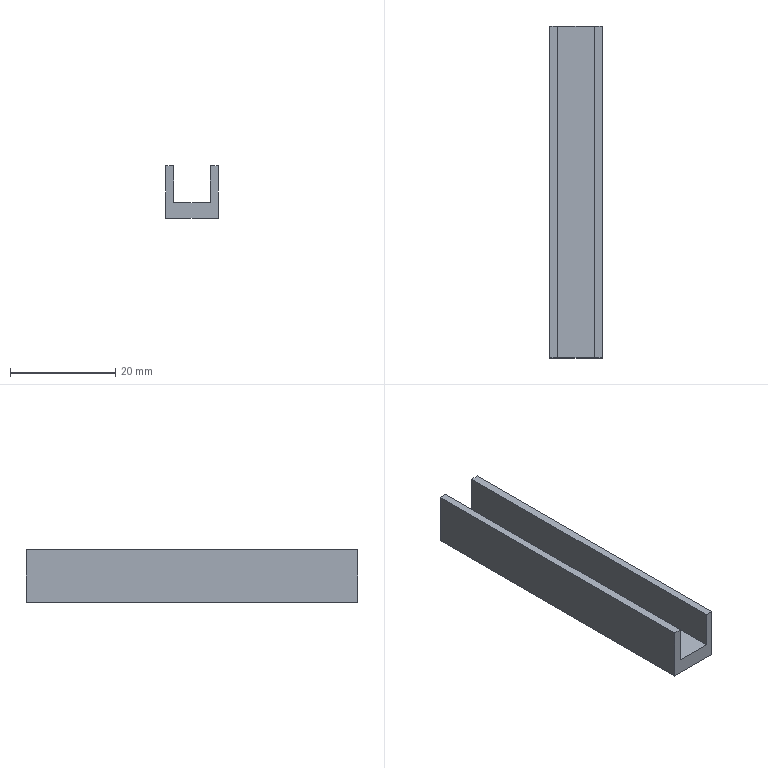Part | STEP file | Magazine box | 1 solid | 10 faces | box 10 x 63 x 10 mm | volume 3213 mm3 | plane 10
STEP:
#1=CARTESIAN_POINT('',(5.,31.5,5.));
#2=VERTEX_POINT('',#1);
#3=CARTESIAN_POINT('',(3.5,31.5,5.));
#4=VERTEX_POINT('',#3);
#5=CARTESIAN_POINT('',(-5.,31.5,5.));
#6=DIRECTION('',(-1.,0.,0.));
#7=VECTOR('',#6,1000.);
#8=LINE('',#5,#7);
#9=EDGE_CURVE('',#2,#4,#8,.T.);
#10=ORIENTED_EDGE('',*,*,#9,.T.);
#11=CARTESIAN_POINT('',(3.5,-31.5,5.));
#12=VERTEX_POINT('',#11);
#13=CARTESIAN_POINT('',(3.5,0.,5.));
#14=DIRECTION('',(0.,-1.,0.));
#15=VECTOR('',#14,1000.);
#16=LINE('',#13,#15);
#17=EDGE_CURVE('',#4,#12,#16,.T.);
#18=ORIENTED_EDGE('',*,*,#17,.T.);
#19=CARTESIAN_POINT('',(5.,-31.5,5.));
#20=VERTEX_POINT('',#19);
#21=CARTESIAN_POINT('',(-5.,-31.5,5.));
#22=DIRECTION('',(1.,0.,0.));
#23=VECTOR('',#22,1000.);
#24=LINE('',#21,#23);
#25=EDGE_CURVE('',#12,#20,#24,.T.);
#26=ORIENTED_EDGE('',*,*,#25,.T.);
#27=CARTESIAN_POINT('',(5.,-31.5,5.));
#28=DIRECTION('',(0.,1.,0.));
#29=VECTOR('',#28,1000.);
#30=LINE('',#27,#29);
#31=EDGE_CURVE('',#20,#2,#30,.T.);
#32=ORIENTED_EDGE('',*,*,#31,.T.);
#33=EDGE_LOOP('',(#10,#18,#26,#32));
#34=FACE_OUTER_BOUND('',#33,.T.);
#35=CARTESIAN_POINT('',(0.,0.,5.));
#36=DIRECTION('',(0.,0.,-1.));
#37=DIRECTION('',(-1.,0.,0.));
#38=AXIS2_PLACEMENT_3D('',#35,#36,#37);
#39=PLANE('',#38);
#40=ADVANCED_FACE('',(#34),#39,.F.);
#41=CARTESIAN_POINT('',(5.,-31.5,-5.));
#42=VERTEX_POINT('',#41);
#43=CARTESIAN_POINT('',(5.,31.5,-5.));
#44=VERTEX_POINT('',#43);
#45=CARTESIAN_POINT('',(5.,-31.5,-5.));
#46=DIRECTION('',(0.,1.,0.));
#47=VECTOR('',#46,1000.);
#48=LINE('',#45,#47);
#49=EDGE_CURVE('',#42,#44,#48,.T.);
#50=ORIENTED_EDGE('',*,*,#49,.T.);
#51=CARTESIAN_POINT('',(5.,31.5,5.));
#52=DIRECTION('',(0.,0.,-1.));
#53=VECTOR('',#52,1000.);
#54=LINE('',#51,#53);
#55=EDGE_CURVE('',#2,#44,#54,.T.);
#56=ORIENTED_EDGE('',*,*,#55,.F.);
#57=ORIENTED_EDGE('',*,*,#31,.F.);
#58=CARTESIAN_POINT('',(5.,-31.5,5.));
#59=DIRECTION('',(0.,0.,-1.));
#60=VECTOR('',#59,1000.);
#61=LINE('',#58,#60);
#62=EDGE_CURVE('',#20,#42,#61,.T.);
#63=ORIENTED_EDGE('',*,*,#62,.T.);
#64=EDGE_LOOP('',(#50,#56,#57,#63));
#65=FACE_OUTER_BOUND('',#64,.T.);
#66=CARTESIAN_POINT('',(5.,-31.5,5.));
#67=DIRECTION('',(-1.,0.,0.));
#68=DIRECTION('',(0.,-1.,0.));
#69=AXIS2_PLACEMENT_3D('',#66,#67,#68);
#70=PLANE('',#69);
#71=ADVANCED_FACE('',(#65),#70,.F.);
#72=CARTESIAN_POINT('',(3.5,31.5,-2.));
#73=VERTEX_POINT('',#72);
#74=CARTESIAN_POINT('',(-3.5,31.5,-2.));
#75=VERTEX_POINT('',#74);
#76=CARTESIAN_POINT('',(-5.,31.5,-2.));
#77=DIRECTION('',(-1.,0.,0.));
#78=VECTOR('',#77,1000.);
#79=LINE('',#76,#78);
#80=EDGE_CURVE('',#73,#75,#79,.T.);
#81=ORIENTED_EDGE('',*,*,#80,.F.);
#82=CARTESIAN_POINT('',(3.5,31.5,5.));
#83=DIRECTION('',(0.,0.,1.));
#84=VECTOR('',#83,1000.);
#85=LINE('',#82,#84);
#86=EDGE_CURVE('',#73,#4,#85,.T.);
#87=ORIENTED_EDGE('',*,*,#86,.T.);
#88=ORIENTED_EDGE('',*,*,#9,.F.);
#89=ORIENTED_EDGE('',*,*,#55,.T.);
#90=CARTESIAN_POINT('',(-5.,31.5,-5.));
#91=VERTEX_POINT('',#90);
#92=CARTESIAN_POINT('',(-5.,31.5,-5.));
#93=DIRECTION('',(-1.,0.,0.));
#94=VECTOR('',#93,1000.);
#95=LINE('',#92,#94);
#96=EDGE_CURVE('',#44,#91,#95,.T.);
#97=ORIENTED_EDGE('',*,*,#96,.T.);
#98=CARTESIAN_POINT('',(-5.,31.5,5.));
#99=VERTEX_POINT('',#98);
#100=CARTESIAN_POINT('',(-5.,31.5,5.));
#101=DIRECTION('',(0.,0.,-1.));
#102=VECTOR('',#101,1000.);
#103=LINE('',#100,#102);
#104=EDGE_CURVE('',#99,#91,#103,.T.);
#105=ORIENTED_EDGE('',*,*,#104,.F.);
#106=CARTESIAN_POINT('',(-3.5,31.5,5.));
#107=VERTEX_POINT('',#106);
#108=CARTESIAN_POINT('',(-5.,31.5,5.));
#109=DIRECTION('',(-1.,0.,0.));
#110=VECTOR('',#109,1000.);
#111=LINE('',#108,#110);
#112=EDGE_CURVE('',#107,#99,#111,.T.);
#113=ORIENTED_EDGE('',*,*,#112,.F.);
#114=CARTESIAN_POINT('',(-3.5,31.5,5.));
#115=DIRECTION('',(0.,0.,-1.));
#116=VECTOR('',#115,1000.);
#117=LINE('',#114,#116);
#118=EDGE_CURVE('',#107,#75,#117,.T.);
#119=ORIENTED_EDGE('',*,*,#118,.T.);
#120=EDGE_LOOP('',(#81,#87,#88,#89,#97,#105,#113,#119));
#121=FACE_OUTER_BOUND('',#120,.T.);
#122=CARTESIAN_POINT('',(-5.,31.5,5.));
#123=DIRECTION('',(0.,-1.,0.));
#124=DIRECTION('',(1.,0.,0.));
#125=AXIS2_PLACEMENT_3D('',#122,#123,#124);
#126=PLANE('',#125);
#127=ADVANCED_FACE('',(#121),#126,.F.);
#128=CARTESIAN_POINT('',(-5.,-31.5,-5.));
#129=VERTEX_POINT('',#128);
#130=CARTESIAN_POINT('',(-5.,-31.5,-5.));
#131=DIRECTION('',(0.,-1.,0.));
#132=VECTOR('',#131,1000.);
#133=LINE('',#130,#132);
#134=EDGE_CURVE('',#91,#129,#133,.T.);
#135=ORIENTED_EDGE('',*,*,#134,.T.);
#136=CARTESIAN_POINT('',(-5.,-31.5,5.));
#137=VERTEX_POINT('',#136);
#138=CARTESIAN_POINT('',(-5.,-31.5,5.));
#139=DIRECTION('',(0.,0.,-1.));
#140=VECTOR('',#139,1000.);
#141=LINE('',#138,#140);
#142=EDGE_CURVE('',#137,#129,#141,.T.);
#143=ORIENTED_EDGE('',*,*,#142,.F.);
#144=CARTESIAN_POINT('',(-5.,-31.5,5.));
#145=DIRECTION('',(0.,-1.,0.));
#146=VECTOR('',#145,1000.);
#147=LINE('',#144,#146);
#148=EDGE_CURVE('',#99,#137,#147,.T.);
#149=ORIENTED_EDGE('',*,*,#148,.F.);
#150=ORIENTED_EDGE('',*,*,#104,.T.);
#151=EDGE_LOOP('',(#135,#143,#149,#150));
#152=FACE_OUTER_BOUND('',#151,.T.);
#153=CARTESIAN_POINT('',(-5.,-31.5,5.));
#154=DIRECTION('',(1.,0.,0.));
#155=DIRECTION('',(0.,0.,-1.));
#156=AXIS2_PLACEMENT_3D('',#153,#154,#155);
#157=PLANE('',#156);
#158=ADVANCED_FACE('',(#152),#157,.F.);
#159=ORIENTED_EDGE('',*,*,#25,.F.);
#160=CARTESIAN_POINT('',(3.5,-31.5,-2.));
#161=VERTEX_POINT('',#160);
#162=CARTESIAN_POINT('',(3.5,-31.5,5.));
#163=DIRECTION('',(0.,0.,-1.));
#164=VECTOR('',#163,1000.);
#165=LINE('',#162,#164);
#166=EDGE_CURVE('',#12,#161,#165,.T.);
#167=ORIENTED_EDGE('',*,*,#166,.T.);
#168=CARTESIAN_POINT('',(-3.5,-31.5,-2.));
#169=VERTEX_POINT('',#168);
#170=CARTESIAN_POINT('',(-5.,-31.5,-2.));
#171=DIRECTION('',(1.,0.,0.));
#172=VECTOR('',#171,1000.);
#173=LINE('',#170,#172);
#174=EDGE_CURVE('',#169,#161,#173,.T.);
#175=ORIENTED_EDGE('',*,*,#174,.F.);
#176=CARTESIAN_POINT('',(-3.5,-31.5,5.));
#177=VERTEX_POINT('',#176);
#178=CARTESIAN_POINT('',(-3.5,-31.5,5.));
#179=DIRECTION('',(0.,0.,1.));
#180=VECTOR('',#179,1000.);
#181=LINE('',#178,#180);
#182=EDGE_CURVE('',#169,#177,#181,.T.);
#183=ORIENTED_EDGE('',*,*,#182,.T.);
#184=CARTESIAN_POINT('',(-5.,-31.5,5.));
#185=DIRECTION('',(1.,0.,0.));
#186=VECTOR('',#185,1000.);
#187=LINE('',#184,#186);
#188=EDGE_CURVE('',#137,#177,#187,.T.);
#189=ORIENTED_EDGE('',*,*,#188,.F.);
#190=ORIENTED_EDGE('',*,*,#142,.T.);
#191=CARTESIAN_POINT('',(-5.,-31.5,-5.));
#192=DIRECTION('',(1.,0.,0.));
#193=VECTOR('',#192,1000.);
#194=LINE('',#191,#193);
#195=EDGE_CURVE('',#129,#42,#194,.T.);
#196=ORIENTED_EDGE('',*,*,#195,.T.);
#197=ORIENTED_EDGE('',*,*,#62,.F.);
#198=EDGE_LOOP('',(#159,#167,#175,#183,#189,#190,#196,#197));
#199=FACE_OUTER_BOUND('',#198,.T.);
#200=CARTESIAN_POINT('',(-5.,-31.5,5.));
#201=DIRECTION('',(0.,1.,0.));
#202=DIRECTION('',(0.,0.,1.));
#203=AXIS2_PLACEMENT_3D('',#200,#201,#202);
#204=PLANE('',#203);
#205=ADVANCED_FACE('',(#199),#204,.F.);
#206=ORIENTED_EDGE('',*,*,#188,.T.);
#207=CARTESIAN_POINT('',(-3.5,0.,5.));
#208=DIRECTION('',(0.,1.,0.));
#209=VECTOR('',#208,1000.);
#210=LINE('',#207,#209);
#211=EDGE_CURVE('',#177,#107,#210,.T.);
#212=ORIENTED_EDGE('',*,*,#211,.T.);
#213=ORIENTED_EDGE('',*,*,#112,.T.);
#214=ORIENTED_EDGE('',*,*,#148,.T.);
#215=EDGE_LOOP('',(#206,#212,#213,#214));
#216=FACE_OUTER_BOUND('',#215,.T.);
#217=CARTESIAN_POINT('',(0.,0.,5.));
#218=DIRECTION('',(0.,0.,-1.));
#219=DIRECTION('',(-1.,0.,0.));
#220=AXIS2_PLACEMENT_3D('',#217,#218,#219);
#221=PLANE('',#220);
#222=ADVANCED_FACE('',(#216),#221,.F.);
#223=ORIENTED_EDGE('',*,*,#49,.F.);
#224=ORIENTED_EDGE('',*,*,#195,.F.);
#225=ORIENTED_EDGE('',*,*,#134,.F.);
#226=ORIENTED_EDGE('',*,*,#96,.F.);
#227=EDGE_LOOP('',(#223,#224,#225,#226));
#228=FACE_OUTER_BOUND('',#227,.T.);
#229=CARTESIAN_POINT('',(0.,0.,-5.));
#230=DIRECTION('',(0.,0.,-1.));
#231=DIRECTION('',(-1.,0.,0.));
#232=AXIS2_PLACEMENT_3D('',#229,#230,#231);
#233=PLANE('',#232);
#234=ADVANCED_FACE('',(#228),#233,.T.);
#235=ORIENTED_EDGE('',*,*,#80,.T.);
#236=CARTESIAN_POINT('',(-3.5,42.509,-2.));
#237=DIRECTION('',(0.,-1.,0.));
#238=VECTOR('',#237,1000.);
#239=LINE('',#236,#238);
#240=EDGE_CURVE('',#75,#169,#239,.T.);
#241=ORIENTED_EDGE('',*,*,#240,.T.);
#242=ORIENTED_EDGE('',*,*,#174,.T.);
#243=CARTESIAN_POINT('',(3.5,42.509,-2.));
#244=DIRECTION('',(0.,1.,0.));
#245=VECTOR('',#244,1000.);
#246=LINE('',#243,#245);
#247=EDGE_CURVE('',#161,#73,#246,.T.);
#248=ORIENTED_EDGE('',*,*,#247,.T.);
#249=EDGE_LOOP('',(#235,#241,#242,#248));
#250=FACE_OUTER_BOUND('',#249,.T.);
#251=CARTESIAN_POINT('',(0.,0.,-2.));
#252=DIRECTION('',(0.,0.,1.));
#253=DIRECTION('',(1.,0.,0.));
#254=AXIS2_PLACEMENT_3D('',#251,#252,#253);
#255=PLANE('',#254);
#256=ADVANCED_FACE('',(#250),#255,.T.);
#257=ORIENTED_EDGE('',*,*,#247,.F.);
#258=ORIENTED_EDGE('',*,*,#166,.F.);
#259=ORIENTED_EDGE('',*,*,#17,.F.);
#260=ORIENTED_EDGE('',*,*,#86,.F.);
#261=EDGE_LOOP('',(#257,#258,#259,#260));
#262=FACE_OUTER_BOUND('',#261,.T.);
#263=CARTESIAN_POINT('',(3.5,42.509,-2.));
#264=DIRECTION('',(1.,0.,0.));
#265=DIRECTION('',(0.,0.,-1.));
#266=AXIS2_PLACEMENT_3D('',#263,#264,#265);
#267=PLANE('',#266);
#268=ADVANCED_FACE('',(#262),#267,.F.);
#269=ORIENTED_EDGE('',*,*,#211,.F.);
#270=ORIENTED_EDGE('',*,*,#182,.F.);
#271=ORIENTED_EDGE('',*,*,#240,.F.);
#272=ORIENTED_EDGE('',*,*,#118,.F.);
#273=EDGE_LOOP('',(#269,#270,#271,#272));
#274=FACE_OUTER_BOUND('',#273,.T.);
#275=CARTESIAN_POINT('',(-3.5,42.509,-2.));
#276=DIRECTION('',(-1.,0.,0.));
#277=DIRECTION('',(0.,0.,1.));
#278=AXIS2_PLACEMENT_3D('',#275,#276,#277);
#279=PLANE('',#278);
#280=ADVANCED_FACE('',(#274),#279,.F.);
#281=CLOSED_SHELL('',(#40,#71,#127,#158,#205,#222,#234,#256,#268,#280));
#282=MANIFOLD_SOLID_BREP('',#281);
#283=CARTESIAN_POINT('',(0.,0.,0.));
#284=DIRECTION('',(0.,0.,1.));
#285=DIRECTION('',(1.,0.,0.));
#286=AXIS2_PLACEMENT_3D('',#283,#284,#285);
#287=(LENGTH_UNIT()NAMED_UNIT(*)SI_UNIT(.MILLI.,.METRE.));
#288=UNCERTAINTY_MEASURE_WITH_UNIT(LENGTH_MEASURE(0.00001),#287,'','');
#289=(NAMED_UNIT(*)PLANE_ANGLE_UNIT()SI_UNIT($,.RADIAN.));
#290=(NAMED_UNIT(*)SI_UNIT($,.STERADIAN.)SOLID_ANGLE_UNIT());
#291=(GEOMETRIC_REPRESENTATION_CONTEXT(3)GLOBAL_UNCERTAINTY_ASSIGNED_CONTEXT((#288))GLOBAL_UNIT_ASSIGNED_CONTEXT((#287,#289,#290))REPRESENTATION_CONTEXT('',''));
#292=ADVANCED_BREP_SHAPE_REPRESENTATION('',(#282,#286),#291);